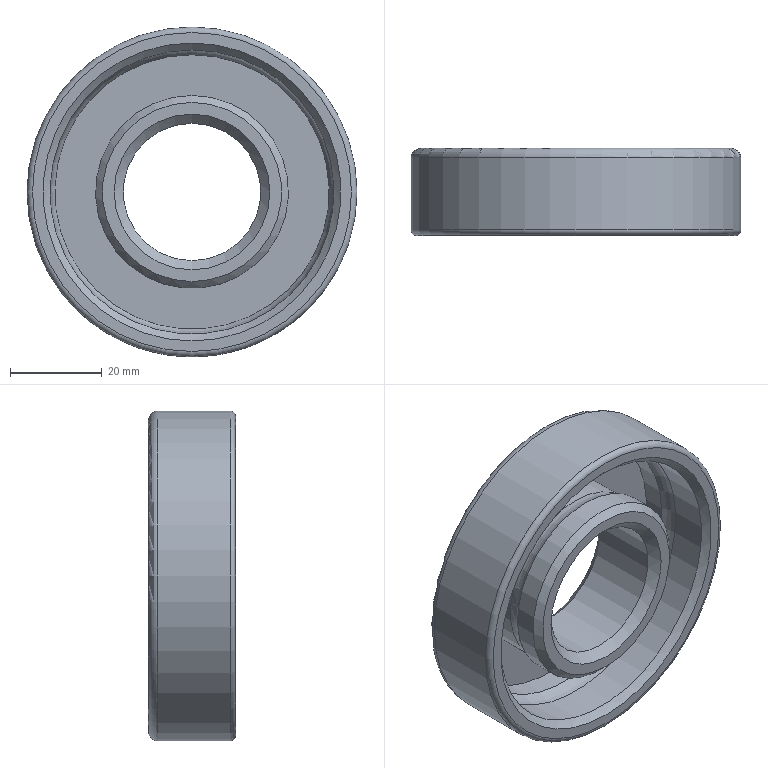Part | NX | features BREP 1, DATUM_CSYS 1 | 1 solid | 22 faces | box 72 x 19 x 72 mm | volume 32783 mm3 | cylinder 6 | cone 6 | plane 6 | torus 4 | commonest cylinder face diameters 30 x1 40 x1 42.101 x1 59.899 x1 62 x1 72 x1
STEP:
#1=CARTESIAN_POINT('',(160.,617.,31.));
#2=VERTEX_POINT('',#1);
#3=CARTESIAN_POINT('',(160.,617.,0.));
#4=DIRECTION('',(0.,1.,0.));
#5=DIRECTION('',(0.,0.,1.));
#6=AXIS2_PLACEMENT_3D('',#3,#4,#5);
#7=CIRCLE('',#6,31.);
#8=EDGE_CURVE('',#2,#2,#7,.F.);
#9=ORIENTED_EDGE('',*,*,#8,.F.);
#10=EDGE_LOOP('',(#9));
#11=FACE_BOUND('',#10,.T.);
#12=CARTESIAN_POINT('',(160.,609.,31.));
#13=VERTEX_POINT('',#12);
#14=CARTESIAN_POINT('',(160.,609.,0.));
#15=DIRECTION('',(0.,1.,0.));
#16=DIRECTION('',(0.,0.,1.));
#17=AXIS2_PLACEMENT_3D('',#14,#15,#16);
#18=CIRCLE('',#17,31.);
#19=EDGE_CURVE('',#13,#13,#18,.F.);
#20=ORIENTED_EDGE('',*,*,#19,.T.);
#21=EDGE_LOOP('',(#20));
#22=FACE_BOUND('',#21,.T.);
#23=CARTESIAN_POINT('',(160.,607.5,0.));
#24=DIRECTION('',(0.,-1.,0.));
#25=DIRECTION('',(0.,0.,1.));
#26=AXIS2_PLACEMENT_3D('',#23,#24,#25);
#27=CYLINDRICAL_SURFACE('',#26,31.);
#28=ADVANCED_FACE('',(#11,#22),#27,.F.);
#29=CARTESIAN_POINT('',(160.,620.233,29.95));
#30=VERTEX_POINT('',#29);
#31=CARTESIAN_POINT('',(160.,620.233,0.));
#32=DIRECTION('',(0.,1.,0.));
#33=DIRECTION('',(0.,0.,1.));
#34=AXIS2_PLACEMENT_3D('',#31,#32,#33);
#35=CIRCLE('',#34,29.95);
#36=EDGE_CURVE('',#30,#30,#35,.F.);
#37=ORIENTED_EDGE('',*,*,#36,.F.);
#38=EDGE_LOOP('',(#37));
#39=FACE_BOUND('',#38,.T.);
#40=ORIENTED_EDGE('',*,*,#8,.T.);
#41=EDGE_LOOP('',(#40));
#42=FACE_BOUND('',#41,.T.);
#43=CARTESIAN_POINT('',(160.,617.,0.));
#44=DIRECTION('',(0.,-1.,0.));
#45=DIRECTION('',(0.,0.,1.));
#46=AXIS2_PLACEMENT_3D('',#43,#44,#45);
#47=TOROIDAL_SURFACE('',#46,25.5,5.5);
#48=ADVANCED_FACE('',(#39,#42),#47,.F.);
#49=CARTESIAN_POINT('',(160.,625.,29.95));
#50=VERTEX_POINT('',#49);
#51=CARTESIAN_POINT('',(160.,625.,0.));
#52=DIRECTION('',(0.,1.,0.));
#53=DIRECTION('',(0.,0.,1.));
#54=AXIS2_PLACEMENT_3D('',#51,#52,#53);
#55=CIRCLE('',#54,29.95);
#56=EDGE_CURVE('',#50,#50,#55,.F.);
#57=ORIENTED_EDGE('',*,*,#56,.F.);
#58=EDGE_LOOP('',(#57));
#59=FACE_BOUND('',#58,.T.);
#60=ORIENTED_EDGE('',*,*,#36,.T.);
#61=EDGE_LOOP('',(#60));
#62=FACE_BOUND('',#61,.T.);
#63=CARTESIAN_POINT('',(160.,607.5,0.));
#64=DIRECTION('',(0.,-1.,0.));
#65=DIRECTION('',(0.,0.,1.));
#66=AXIS2_PLACEMENT_3D('',#63,#64,#65);
#67=CYLINDRICAL_SURFACE('',#66,29.95);
#68=ADVANCED_FACE('',(#59,#62),#67,.F.);
#69=CARTESIAN_POINT('',(160.,625.75,30.7));
#70=VERTEX_POINT('',#69);
#71=CARTESIAN_POINT('',(160.,625.75,0.));
#72=DIRECTION('',(0.,1.,0.));
#73=DIRECTION('',(0.,0.,1.));
#74=AXIS2_PLACEMENT_3D('',#71,#72,#73);
#75=CIRCLE('',#74,30.7);
#76=EDGE_CURVE('',#70,#70,#75,.F.);
#77=ORIENTED_EDGE('',*,*,#76,.T.);
#78=EDGE_LOOP('',(#77));
#79=FACE_BOUND('',#78,.T.);
#80=CARTESIAN_POINT('',(160.,626.5,31.45));
#81=VERTEX_POINT('',#80);
#82=CARTESIAN_POINT('',(160.,626.5,0.));
#83=DIRECTION('',(0.,1.,0.));
#84=DIRECTION('',(0.,0.,1.));
#85=AXIS2_PLACEMENT_3D('',#82,#83,#84);
#86=CIRCLE('',#85,31.45);
#87=EDGE_CURVE('',#81,#81,#86,.F.);
#88=ORIENTED_EDGE('',*,*,#87,.F.);
#89=EDGE_LOOP('',(#88));
#90=FACE_BOUND('',#89,.T.);
#91=CARTESIAN_POINT('',(160.,625.,0.));
#92=DIRECTION('',(0.,1.,0.));
#93=DIRECTION('',(0.,0.,-1.));
#94=AXIS2_PLACEMENT_3D('',#91,#92,#93);
#95=CONICAL_SURFACE('',#94,29.95,0.7854);
#96=ADVANCED_FACE('',(#79,#90),#95,.F.);
#97=CARTESIAN_POINT('',(160.,626.5,34.));
#98=VERTEX_POINT('',#97);
#99=CARTESIAN_POINT('',(160.,626.5,0.));
#100=DIRECTION('',(0.,1.,0.));
#101=DIRECTION('',(0.,0.,1.));
#102=AXIS2_PLACEMENT_3D('',#99,#100,#101);
#103=CIRCLE('',#102,34.);
#104=EDGE_CURVE('',#98,#98,#103,.F.);
#105=ORIENTED_EDGE('',*,*,#104,.F.);
#106=EDGE_LOOP('',(#105));
#107=FACE_BOUND('',#106,.T.);
#108=ORIENTED_EDGE('',*,*,#87,.T.);
#109=EDGE_LOOP('',(#108));
#110=FACE_BOUND('',#109,.T.);
#111=CARTESIAN_POINT('',(128.55,626.5,0.));
#112=DIRECTION('',(0.,-1.,0.));
#113=DIRECTION('',(0.,0.,1.));
#114=AXIS2_PLACEMENT_3D('',#111,#112,#113);
#115=PLANE('',#114);
#116=ADVANCED_FACE('',(#107,#110),#115,.F.);
#117=CARTESIAN_POINT('',(160.,624.5,36.));
#118=VERTEX_POINT('',#117);
#119=CARTESIAN_POINT('',(160.,624.5,0.));
#120=DIRECTION('',(0.,1.,0.));
#121=DIRECTION('',(0.,0.,1.));
#122=AXIS2_PLACEMENT_3D('',#119,#120,#121);
#123=CIRCLE('',#122,36.);
#124=EDGE_CURVE('',#118,#118,#123,.F.);
#125=ORIENTED_EDGE('',*,*,#124,.F.);
#126=EDGE_LOOP('',(#125));
#127=FACE_BOUND('',#126,.T.);
#128=ORIENTED_EDGE('',*,*,#104,.T.);
#129=EDGE_LOOP('',(#128));
#130=FACE_BOUND('',#129,.T.);
#131=CARTESIAN_POINT('',(160.,624.5,0.));
#132=DIRECTION('',(0.,-1.,0.));
#133=DIRECTION('',(0.,0.,1.));
#134=AXIS2_PLACEMENT_3D('',#131,#132,#133);
#135=TOROIDAL_SURFACE('',#134,34.,2.);
#136=ADVANCED_FACE('',(#127,#130),#135,.T.);
#137=CARTESIAN_POINT('',(160.,608.7,36.));
#138=VERTEX_POINT('',#137);
#139=CARTESIAN_POINT('',(160.,608.7,0.));
#140=DIRECTION('',(0.,1.,0.));
#141=DIRECTION('',(0.,0.,1.));
#142=AXIS2_PLACEMENT_3D('',#139,#140,#141);
#143=CIRCLE('',#142,36.);
#144=EDGE_CURVE('',#138,#138,#143,.F.);
#145=ORIENTED_EDGE('',*,*,#144,.F.);
#146=EDGE_LOOP('',(#145));
#147=FACE_BOUND('',#146,.T.);
#148=ORIENTED_EDGE('',*,*,#124,.T.);
#149=EDGE_LOOP('',(#148));
#150=FACE_BOUND('',#149,.T.);
#151=CARTESIAN_POINT('',(160.,607.5,0.));
#152=DIRECTION('',(0.,-1.,0.));
#153=DIRECTION('',(0.,0.,1.));
#154=AXIS2_PLACEMENT_3D('',#151,#152,#153);
#155=CYLINDRICAL_SURFACE('',#154,36.);
#156=ADVANCED_FACE('',(#147,#150),#155,.T.);
#157=CARTESIAN_POINT('',(160.,607.5,34.8));
#158=VERTEX_POINT('',#157);
#159=CARTESIAN_POINT('',(160.,607.5,0.));
#160=DIRECTION('',(0.,1.,0.));
#161=DIRECTION('',(0.,0.,1.));
#162=AXIS2_PLACEMENT_3D('',#159,#160,#161);
#163=CIRCLE('',#162,34.8);
#164=EDGE_CURVE('',#158,#158,#163,.F.);
#165=ORIENTED_EDGE('',*,*,#164,.F.);
#166=EDGE_LOOP('',(#165));
#167=FACE_BOUND('',#166,.T.);
#168=ORIENTED_EDGE('',*,*,#144,.T.);
#169=EDGE_LOOP('',(#168));
#170=FACE_BOUND('',#169,.T.);
#171=CARTESIAN_POINT('',(160.,608.7,0.));
#172=DIRECTION('',(0.,-1.,0.));
#173=DIRECTION('',(0.,0.,1.));
#174=AXIS2_PLACEMENT_3D('',#171,#172,#173);
#175=TOROIDAL_SURFACE('',#174,34.8,1.2);
#176=ADVANCED_FACE('',(#167,#170),#175,.T.);
#177=CARTESIAN_POINT('',(160.,607.5,32.5));
#178=VERTEX_POINT('',#177);
#179=CARTESIAN_POINT('',(160.,607.5,0.));
#180=DIRECTION('',(0.,1.,0.));
#181=DIRECTION('',(0.,0.,1.));
#182=AXIS2_PLACEMENT_3D('',#179,#180,#181);
#183=CIRCLE('',#182,32.5);
#184=EDGE_CURVE('',#178,#178,#183,.F.);
#185=ORIENTED_EDGE('',*,*,#184,.F.);
#186=EDGE_LOOP('',(#185));
#187=FACE_BOUND('',#186,.T.);
#188=ORIENTED_EDGE('',*,*,#164,.T.);
#189=EDGE_LOOP('',(#188));
#190=FACE_BOUND('',#189,.T.);
#191=CARTESIAN_POINT('',(125.2,607.5,0.));
#192=DIRECTION('',(0.,1.,0.));
#193=DIRECTION('',(0.,0.,-1.));
#194=AXIS2_PLACEMENT_3D('',#191,#192,#193);
#195=PLANE('',#194);
#196=ADVANCED_FACE('',(#187,#190),#195,.F.);
#197=ORIENTED_EDGE('',*,*,#19,.F.);
#198=EDGE_LOOP('',(#197));
#199=FACE_BOUND('',#198,.T.);
#200=ORIENTED_EDGE('',*,*,#184,.T.);
#201=EDGE_LOOP('',(#200));
#202=FACE_BOUND('',#201,.T.);
#203=CARTESIAN_POINT('',(160.,607.5,0.));
#204=DIRECTION('',(0.,-1.,0.));
#205=DIRECTION('',(0.,0.,1.));
#206=AXIS2_PLACEMENT_3D('',#203,#204,#205);
#207=CONICAL_SURFACE('',#206,32.5,0.7854);
#208=ADVANCED_FACE('',(#199,#202),#207,.F.);
#209=CARTESIAN_POINT('',(160.,626.5,18.5));
#210=VERTEX_POINT('',#209);
#211=CARTESIAN_POINT('',(160.,626.5,0.));
#212=DIRECTION('',(0.,1.,0.));
#213=DIRECTION('',(0.,0.,1.));
#214=AXIS2_PLACEMENT_3D('',#211,#212,#213);
#215=CIRCLE('',#214,18.5);
#216=EDGE_CURVE('',#210,#210,#215,.F.);
#217=ORIENTED_EDGE('',*,*,#216,.T.);
#218=EDGE_LOOP('',(#217));
#219=FACE_BOUND('',#218,.T.);
#220=CARTESIAN_POINT('',(160.,625.75,19.25));
#221=VERTEX_POINT('',#220);
#222=CARTESIAN_POINT('',(160.,625.75,0.));
#223=DIRECTION('',(0.,1.,0.));
#224=DIRECTION('',(0.,0.,1.));
#225=AXIS2_PLACEMENT_3D('',#222,#223,#224);
#226=CIRCLE('',#225,19.25);
#227=EDGE_CURVE('',#221,#221,#226,.F.);
#228=ORIENTED_EDGE('',*,*,#227,.F.);
#229=EDGE_LOOP('',(#228));
#230=FACE_BOUND('',#229,.T.);
#231=CARTESIAN_POINT('',(160.,626.5,0.));
#232=DIRECTION('',(0.,-1.,0.));
#233=DIRECTION('',(0.,0.,1.));
#234=AXIS2_PLACEMENT_3D('',#231,#232,#233);
#235=CONICAL_SURFACE('',#234,18.5,0.7854);
#236=ADVANCED_FACE('',(#219,#230),#235,.T.);
#237=CARTESIAN_POINT('',(160.,607.5,19.55));
#238=VERTEX_POINT('',#237);
#239=CARTESIAN_POINT('',(160.,607.5,0.));
#240=DIRECTION('',(0.,1.,0.));
#241=DIRECTION('',(0.,0.,1.));
#242=AXIS2_PLACEMENT_3D('',#239,#240,#241);
#243=CIRCLE('',#242,19.55);
#244=EDGE_CURVE('',#238,#238,#243,.F.);
#245=ORIENTED_EDGE('',*,*,#244,.F.);
#246=EDGE_LOOP('',(#245));
#247=FACE_BOUND('',#246,.T.);
#248=CARTESIAN_POINT('',(160.,609.,21.05));
#249=VERTEX_POINT('',#248);
#250=CARTESIAN_POINT('',(160.,609.,0.));
#251=DIRECTION('',(0.,1.,0.));
#252=DIRECTION('',(0.,0.,1.));
#253=AXIS2_PLACEMENT_3D('',#250,#251,#252);
#254=CIRCLE('',#253,21.05);
#255=EDGE_CURVE('',#249,#249,#254,.F.);
#256=ORIENTED_EDGE('',*,*,#255,.T.);
#257=EDGE_LOOP('',(#256));
#258=FACE_BOUND('',#257,.T.);
#259=CARTESIAN_POINT('',(160.,609.,0.));
#260=DIRECTION('',(0.,1.,0.));
#261=DIRECTION('',(0.,0.,-1.));
#262=AXIS2_PLACEMENT_3D('',#259,#260,#261);
#263=CONICAL_SURFACE('',#262,21.05,0.7854);
#264=ADVANCED_FACE('',(#247,#258),#263,.T.);
#265=CARTESIAN_POINT('',(160.,607.5,17.));
#266=VERTEX_POINT('',#265);
#267=CARTESIAN_POINT('',(160.,607.5,0.));
#268=DIRECTION('',(0.,1.,0.));
#269=DIRECTION('',(0.,0.,1.));
#270=AXIS2_PLACEMENT_3D('',#267,#268,#269);
#271=CIRCLE('',#270,17.);
#272=EDGE_CURVE('',#266,#266,#271,.F.);
#273=ORIENTED_EDGE('',*,*,#272,.F.);
#274=EDGE_LOOP('',(#273));
#275=FACE_BOUND('',#274,.T.);
#276=ORIENTED_EDGE('',*,*,#244,.T.);
#277=EDGE_LOOP('',(#276));
#278=FACE_BOUND('',#277,.T.);
#279=CARTESIAN_POINT('',(140.45,607.5,0.));
#280=DIRECTION('',(0.,1.,0.));
#281=DIRECTION('',(0.,0.,-1.));
#282=AXIS2_PLACEMENT_3D('',#279,#280,#281);
#283=PLANE('',#282);
#284=ADVANCED_FACE('',(#275,#278),#283,.F.);
#285=CARTESIAN_POINT('',(160.,609.5,15.));
#286=VERTEX_POINT('',#285);
#287=CARTESIAN_POINT('',(160.,609.5,0.));
#288=DIRECTION('',(0.,1.,0.));
#289=DIRECTION('',(0.,0.,1.));
#290=AXIS2_PLACEMENT_3D('',#287,#288,#289);
#291=CIRCLE('',#290,15.);
#292=EDGE_CURVE('',#286,#286,#291,.F.);
#293=ORIENTED_EDGE('',*,*,#292,.F.);
#294=EDGE_LOOP('',(#293));
#295=FACE_BOUND('',#294,.T.);
#296=ORIENTED_EDGE('',*,*,#272,.T.);
#297=EDGE_LOOP('',(#296));
#298=FACE_BOUND('',#297,.T.);
#299=CARTESIAN_POINT('',(160.,607.5,0.));
#300=DIRECTION('',(0.,-1.,0.));
#301=DIRECTION('',(0.,0.,1.));
#302=AXIS2_PLACEMENT_3D('',#299,#300,#301);
#303=CONICAL_SURFACE('',#302,17.,0.7854);
#304=ADVANCED_FACE('',(#295,#298),#303,.F.);
#305=CARTESIAN_POINT('',(160.,624.5,15.));
#306=VERTEX_POINT('',#305);
#307=CARTESIAN_POINT('',(160.,624.5,0.));
#308=DIRECTION('',(0.,1.,0.));
#309=DIRECTION('',(0.,0.,1.));
#310=AXIS2_PLACEMENT_3D('',#307,#308,#309);
#311=CIRCLE('',#310,15.);
#312=EDGE_CURVE('',#306,#306,#311,.F.);
#313=ORIENTED_EDGE('',*,*,#312,.F.);
#314=EDGE_LOOP('',(#313));
#315=FACE_BOUND('',#314,.T.);
#316=ORIENTED_EDGE('',*,*,#292,.T.);
#317=EDGE_LOOP('',(#316));
#318=FACE_BOUND('',#317,.T.);
#319=CARTESIAN_POINT('',(160.,607.5,0.));
#320=DIRECTION('',(0.,-1.,0.));
#321=DIRECTION('',(0.,0.,1.));
#322=AXIS2_PLACEMENT_3D('',#319,#320,#321);
#323=CYLINDRICAL_SURFACE('',#322,15.);
#324=ADVANCED_FACE('',(#315,#318),#323,.F.);
#325=CARTESIAN_POINT('',(160.,626.5,17.));
#326=VERTEX_POINT('',#325);
#327=CARTESIAN_POINT('',(160.,626.5,0.));
#328=DIRECTION('',(0.,1.,0.));
#329=DIRECTION('',(0.,0.,1.));
#330=AXIS2_PLACEMENT_3D('',#327,#328,#329);
#331=CIRCLE('',#330,17.);
#332=EDGE_CURVE('',#326,#326,#331,.F.);
#333=ORIENTED_EDGE('',*,*,#332,.F.);
#334=EDGE_LOOP('',(#333));
#335=FACE_BOUND('',#334,.T.);
#336=ORIENTED_EDGE('',*,*,#312,.T.);
#337=EDGE_LOOP('',(#336));
#338=FACE_BOUND('',#337,.T.);
#339=CARTESIAN_POINT('',(160.,624.5,0.));
#340=DIRECTION('',(0.,1.,0.));
#341=DIRECTION('',(0.,0.,-1.));
#342=AXIS2_PLACEMENT_3D('',#339,#340,#341);
#343=CONICAL_SURFACE('',#342,15.,0.7854);
#344=ADVANCED_FACE('',(#335,#338),#343,.F.);
#345=ORIENTED_EDGE('',*,*,#216,.F.);
#346=EDGE_LOOP('',(#345));
#347=FACE_BOUND('',#346,.T.);
#348=ORIENTED_EDGE('',*,*,#332,.T.);
#349=EDGE_LOOP('',(#348));
#350=FACE_BOUND('',#349,.T.);
#351=CARTESIAN_POINT('',(143.,626.5,0.));
#352=DIRECTION('',(0.,-1.,0.));
#353=DIRECTION('',(0.,0.,1.));
#354=AXIS2_PLACEMENT_3D('',#351,#352,#353);
#355=PLANE('',#354);
#356=ADVANCED_FACE('',(#347,#350),#355,.F.);
#357=CARTESIAN_POINT('',(160.,617.,20.));
#358=VERTEX_POINT('',#357);
#359=CARTESIAN_POINT('',(160.,617.,0.));
#360=DIRECTION('',(0.,1.,0.));
#361=DIRECTION('',(0.,0.,1.));
#362=AXIS2_PLACEMENT_3D('',#359,#360,#361);
#363=CIRCLE('',#362,20.);
#364=EDGE_CURVE('',#358,#358,#363,.F.);
#365=ORIENTED_EDGE('',*,*,#364,.F.);
#366=EDGE_LOOP('',(#365));
#367=FACE_BOUND('',#366,.T.);
#368=CARTESIAN_POINT('',(160.,625.,20.));
#369=VERTEX_POINT('',#368);
#370=CARTESIAN_POINT('',(160.,625.,0.));
#371=DIRECTION('',(0.,1.,0.));
#372=DIRECTION('',(0.,0.,1.));
#373=AXIS2_PLACEMENT_3D('',#370,#371,#372);
#374=CIRCLE('',#373,20.);
#375=EDGE_CURVE('',#369,#369,#374,.F.);
#376=ORIENTED_EDGE('',*,*,#375,.T.);
#377=EDGE_LOOP('',(#376));
#378=FACE_BOUND('',#377,.T.);
#379=CARTESIAN_POINT('',(160.,607.5,0.));
#380=DIRECTION('',(0.,-1.,0.));
#381=DIRECTION('',(0.,0.,1.));
#382=AXIS2_PLACEMENT_3D('',#379,#380,#381);
#383=CYLINDRICAL_SURFACE('',#382,20.);
#384=ADVANCED_FACE('',(#367,#378),#383,.T.);
#385=CARTESIAN_POINT('',(160.,613.767,21.05));
#386=VERTEX_POINT('',#385);
#387=CARTESIAN_POINT('',(160.,613.767,0.));
#388=DIRECTION('',(0.,1.,0.));
#389=DIRECTION('',(0.,0.,1.));
#390=AXIS2_PLACEMENT_3D('',#387,#388,#389);
#391=CIRCLE('',#390,21.05);
#392=EDGE_CURVE('',#386,#386,#391,.F.);
#393=ORIENTED_EDGE('',*,*,#392,.F.);
#394=EDGE_LOOP('',(#393));
#395=FACE_BOUND('',#394,.T.);
#396=ORIENTED_EDGE('',*,*,#364,.T.);
#397=EDGE_LOOP('',(#396));
#398=FACE_BOUND('',#397,.T.);
#399=CARTESIAN_POINT('',(160.,617.,0.));
#400=DIRECTION('',(0.,-1.,0.));
#401=DIRECTION('',(0.,0.,1.));
#402=AXIS2_PLACEMENT_3D('',#399,#400,#401);
#403=TOROIDAL_SURFACE('',#402,25.5,5.5);
#404=ADVANCED_FACE('',(#395,#398),#403,.F.);
#405=ORIENTED_EDGE('',*,*,#255,.F.);
#406=EDGE_LOOP('',(#405));
#407=FACE_BOUND('',#406,.T.);
#408=ORIENTED_EDGE('',*,*,#392,.T.);
#409=EDGE_LOOP('',(#408));
#410=FACE_BOUND('',#409,.T.);
#411=CARTESIAN_POINT('',(160.,607.5,0.));
#412=DIRECTION('',(0.,-1.,0.));
#413=DIRECTION('',(0.,0.,1.));
#414=AXIS2_PLACEMENT_3D('',#411,#412,#413);
#415=CYLINDRICAL_SURFACE('',#414,21.05);
#416=ADVANCED_FACE('',(#407,#410),#415,.T.);
#417=ORIENTED_EDGE('',*,*,#375,.F.);
#418=EDGE_LOOP('',(#417));
#419=FACE_BOUND('',#418,.T.);
#420=ORIENTED_EDGE('',*,*,#56,.T.);
#421=EDGE_LOOP('',(#420));
#422=FACE_BOUND('',#421,.T.);
#423=CARTESIAN_POINT('',(130.05,625.,0.));
#424=DIRECTION('',(0.,1.,0.));
#425=DIRECTION('',(0.,0.,-1.));
#426=AXIS2_PLACEMENT_3D('',#423,#424,#425);
#427=PLANE('',#426);
#428=ADVANCED_FACE('',(#419,#422),#427,.F.);
#429=ORIENTED_EDGE('',*,*,#76,.F.);
#430=EDGE_LOOP('',(#429));
#431=FACE_BOUND('',#430,.T.);
#432=ORIENTED_EDGE('',*,*,#227,.T.);
#433=EDGE_LOOP('',(#432));
#434=FACE_BOUND('',#433,.T.);
#435=CARTESIAN_POINT('',(140.75,625.75,0.));
#436=DIRECTION('',(0.,-1.,0.));
#437=DIRECTION('',(0.,0.,1.));
#438=AXIS2_PLACEMENT_3D('',#435,#436,#437);
#439=PLANE('',#438);
#440=ADVANCED_FACE('',(#431,#434),#439,.F.);
#441=CLOSED_SHELL('',(#28,#48,#68,#96,#116,#136,#156,#176,#196,#208,#236,#264,#284,#304,#324,#344,#356,#384,#404,#416,#428,#440));
#442=MANIFOLD_SOLID_BREP('',#441);
#443=(LENGTH_UNIT()NAMED_UNIT(*)SI_UNIT(.MILLI.,.METRE.));
#444=UNCERTAINTY_MEASURE_WITH_UNIT(LENGTH_MEASURE(0.00001),#443,'','');
#445=(NAMED_UNIT(*)PLANE_ANGLE_UNIT()SI_UNIT($,.RADIAN.));
#446=(NAMED_UNIT(*)SI_UNIT($,.STERADIAN.)SOLID_ANGLE_UNIT());
#447=(GEOMETRIC_REPRESENTATION_CONTEXT(3)GLOBAL_UNCERTAINTY_ASSIGNED_CONTEXT((#444))GLOBAL_UNIT_ASSIGNED_CONTEXT((#443,#445,#446))REPRESENTATION_CONTEXT('',''));
#448=ADVANCED_BREP_SHAPE_REPRESENTATION('',(#442),#447);